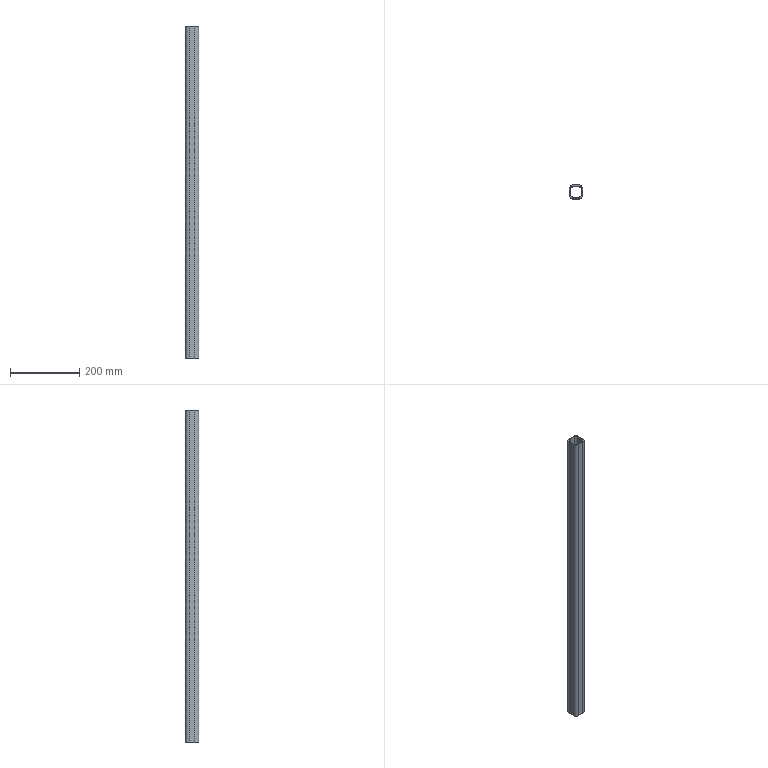Part | SolidWorks | features BaseBody 1 | 1 solid | 18 faces | box 40 x 40 x 962 mm | volume 488049 mm3 | plane 10 | cylinder 8 | commonest cylinder face diameters 16 x4 24 x4
STEP:
#1=CARTESIAN_POINT('',(8.,-20.,-50.));
#2=VERTEX_POINT('',#1);
#3=CARTESIAN_POINT('',(20.,-8.,-50.));
#4=VERTEX_POINT('',#3);
#5=CARTESIAN_POINT('',(8.,-8.,-50.));
#6=DIRECTION('',(0.,0.,1.));
#7=DIRECTION('',(1.,0.,0.));
#8=AXIS2_PLACEMENT_3D('',#5,#6,#7);
#9=CIRCLE('',#8,12.);
#10=EDGE_CURVE('',#2,#4,#9,.T.);
#11=ORIENTED_EDGE('',*,*,#10,.T.);
#12=CARTESIAN_POINT('',(20.,-8.,912.));
#13=VERTEX_POINT('',#12);
#14=CARTESIAN_POINT('',(20.,-8.,0.));
#15=DIRECTION('',(0.,0.,1.));
#16=VECTOR('',#15,1000.);
#17=LINE('',#14,#16);
#18=EDGE_CURVE('',#4,#13,#17,.T.);
#19=ORIENTED_EDGE('',*,*,#18,.T.);
#20=CARTESIAN_POINT('',(8.,-20.,912.));
#21=VERTEX_POINT('',#20);
#22=CARTESIAN_POINT('',(8.,-8.,912.));
#23=DIRECTION('',(0.,0.,-1.));
#24=DIRECTION('',(1.,0.,0.));
#25=AXIS2_PLACEMENT_3D('',#22,#23,#24);
#26=CIRCLE('',#25,12.);
#27=EDGE_CURVE('',#13,#21,#26,.T.);
#28=ORIENTED_EDGE('',*,*,#27,.T.);
#29=CARTESIAN_POINT('',(8.,-20.,0.));
#30=DIRECTION('',(0.,0.,-1.));
#31=VECTOR('',#30,1000.);
#32=LINE('',#29,#31);
#33=EDGE_CURVE('',#21,#2,#32,.T.);
#34=ORIENTED_EDGE('',*,*,#33,.T.);
#35=EDGE_LOOP('',(#11,#19,#28,#34));
#36=FACE_OUTER_BOUND('',#35,.T.);
#37=CARTESIAN_POINT('',(8.,-8.,0.));
#38=DIRECTION('',(0.,0.,1.));
#39=DIRECTION('',(1.,0.,0.));
#40=AXIS2_PLACEMENT_3D('',#37,#38,#39);
#41=CYLINDRICAL_SURFACE('',#40,12.);
#42=ADVANCED_FACE('',(#36),#41,.T.);
#43=CARTESIAN_POINT('',(20.,8.,-50.));
#44=VERTEX_POINT('',#43);
#45=CARTESIAN_POINT('',(20.,8.,-50.));
#46=DIRECTION('',(0.,1.,0.));
#47=VECTOR('',#46,1000.);
#48=LINE('',#45,#47);
#49=EDGE_CURVE('',#4,#44,#48,.T.);
#50=ORIENTED_EDGE('',*,*,#49,.T.);
#51=CARTESIAN_POINT('',(20.,8.,912.));
#52=VERTEX_POINT('',#51);
#53=CARTESIAN_POINT('',(20.,8.,0.));
#54=DIRECTION('',(0.,0.,1.));
#55=VECTOR('',#54,1000.);
#56=LINE('',#53,#55);
#57=EDGE_CURVE('',#44,#52,#56,.T.);
#58=ORIENTED_EDGE('',*,*,#57,.T.);
#59=CARTESIAN_POINT('',(20.,8.,912.));
#60=DIRECTION('',(0.,-1.,0.));
#61=VECTOR('',#60,1000.);
#62=LINE('',#59,#61);
#63=EDGE_CURVE('',#52,#13,#62,.T.);
#64=ORIENTED_EDGE('',*,*,#63,.T.);
#65=ORIENTED_EDGE('',*,*,#18,.F.);
#66=EDGE_LOOP('',(#50,#58,#64,#65));
#67=FACE_OUTER_BOUND('',#66,.T.);
#68=CARTESIAN_POINT('',(20.,8.,0.));
#69=DIRECTION('',(1.,0.,0.));
#70=DIRECTION('',(0.,1.,0.));
#71=AXIS2_PLACEMENT_3D('',#68,#69,#70);
#72=PLANE('',#71);
#73=ADVANCED_FACE('',(#67),#72,.T.);
#74=CARTESIAN_POINT('',(-16.,8.,-50.));
#75=VERTEX_POINT('',#74);
#76=CARTESIAN_POINT('',(-8.,16.,-50.));
#77=VERTEX_POINT('',#76);
#78=CARTESIAN_POINT('',(-8.,8.,-50.));
#79=DIRECTION('',(0.,0.,-1.));
#80=DIRECTION('',(1.,0.,0.));
#81=AXIS2_PLACEMENT_3D('',#78,#79,#80);
#82=CIRCLE('',#81,8.);
#83=EDGE_CURVE('',#75,#77,#82,.T.);
#84=ORIENTED_EDGE('',*,*,#83,.F.);
#85=CARTESIAN_POINT('',(-16.,-8.,-50.));
#86=VERTEX_POINT('',#85);
#87=CARTESIAN_POINT('',(-16.,0.,-50.));
#88=DIRECTION('',(0.,1.,0.));
#89=VECTOR('',#88,1000.);
#90=LINE('',#87,#89);
#91=EDGE_CURVE('',#86,#75,#90,.T.);
#92=ORIENTED_EDGE('',*,*,#91,.F.);
#93=CARTESIAN_POINT('',(-8.,-16.,-50.));
#94=VERTEX_POINT('',#93);
#95=CARTESIAN_POINT('',(-8.,-8.,-50.));
#96=DIRECTION('',(0.,0.,-1.));
#97=DIRECTION('',(1.,0.,0.));
#98=AXIS2_PLACEMENT_3D('',#95,#96,#97);
#99=CIRCLE('',#98,8.);
#100=EDGE_CURVE('',#94,#86,#99,.T.);
#101=ORIENTED_EDGE('',*,*,#100,.F.);
#102=CARTESIAN_POINT('',(8.,-16.,-50.));
#103=VERTEX_POINT('',#102);
#104=CARTESIAN_POINT('',(0.,-16.,-50.));
#105=DIRECTION('',(-1.,0.,0.));
#106=VECTOR('',#105,1000.);
#107=LINE('',#104,#106);
#108=EDGE_CURVE('',#103,#94,#107,.T.);
#109=ORIENTED_EDGE('',*,*,#108,.F.);
#110=CARTESIAN_POINT('',(16.,-8.,-50.));
#111=VERTEX_POINT('',#110);
#112=CARTESIAN_POINT('',(8.,-8.,-50.));
#113=DIRECTION('',(0.,0.,-1.));
#114=DIRECTION('',(1.,0.,0.));
#115=AXIS2_PLACEMENT_3D('',#112,#113,#114);
#116=CIRCLE('',#115,8.);
#117=EDGE_CURVE('',#111,#103,#116,.T.);
#118=ORIENTED_EDGE('',*,*,#117,.F.);
#119=CARTESIAN_POINT('',(16.,8.,-50.));
#120=VERTEX_POINT('',#119);
#121=CARTESIAN_POINT('',(16.,0.,-50.));
#122=DIRECTION('',(0.,-1.,0.));
#123=VECTOR('',#122,1000.);
#124=LINE('',#121,#123);
#125=EDGE_CURVE('',#120,#111,#124,.T.);
#126=ORIENTED_EDGE('',*,*,#125,.F.);
#127=CARTESIAN_POINT('',(8.,16.,-50.));
#128=VERTEX_POINT('',#127);
#129=CARTESIAN_POINT('',(8.,8.,-50.));
#130=DIRECTION('',(0.,0.,-1.));
#131=DIRECTION('',(1.,0.,0.));
#132=AXIS2_PLACEMENT_3D('',#129,#130,#131);
#133=CIRCLE('',#132,8.);
#134=EDGE_CURVE('',#128,#120,#133,.T.);
#135=ORIENTED_EDGE('',*,*,#134,.F.);
#136=CARTESIAN_POINT('',(0.,16.,-50.));
#137=DIRECTION('',(1.,0.,0.));
#138=VECTOR('',#137,1000.);
#139=LINE('',#136,#138);
#140=EDGE_CURVE('',#77,#128,#139,.T.);
#141=ORIENTED_EDGE('',*,*,#140,.F.);
#142=EDGE_LOOP('',(#84,#92,#101,#109,#118,#126,#135,#141));
#143=FACE_BOUND('',#142,.T.);
#144=CARTESIAN_POINT('',(-8.,20.,-50.));
#145=VERTEX_POINT('',#144);
#146=CARTESIAN_POINT('',(-20.,8.,-50.));
#147=VERTEX_POINT('',#146);
#148=CARTESIAN_POINT('',(-8.,8.,-50.));
#149=DIRECTION('',(0.,0.,1.));
#150=DIRECTION('',(1.,0.,0.));
#151=AXIS2_PLACEMENT_3D('',#148,#149,#150);
#152=CIRCLE('',#151,12.);
#153=EDGE_CURVE('',#145,#147,#152,.T.);
#154=ORIENTED_EDGE('',*,*,#153,.F.);
#155=CARTESIAN_POINT('',(8.,20.,-50.));
#156=VERTEX_POINT('',#155);
#157=CARTESIAN_POINT('',(0.,20.,-50.));
#158=DIRECTION('',(-1.,0.,0.));
#159=VECTOR('',#158,1000.);
#160=LINE('',#157,#159);
#161=EDGE_CURVE('',#156,#145,#160,.T.);
#162=ORIENTED_EDGE('',*,*,#161,.F.);
#163=CARTESIAN_POINT('',(8.,8.,-50.));
#164=DIRECTION('',(0.,0.,1.));
#165=DIRECTION('',(1.,0.,0.));
#166=AXIS2_PLACEMENT_3D('',#163,#164,#165);
#167=CIRCLE('',#166,12.);
#168=EDGE_CURVE('',#44,#156,#167,.T.);
#169=ORIENTED_EDGE('',*,*,#168,.F.);
#170=ORIENTED_EDGE('',*,*,#49,.F.);
#171=ORIENTED_EDGE('',*,*,#10,.F.);
#172=CARTESIAN_POINT('',(-8.,-20.,-50.));
#173=VERTEX_POINT('',#172);
#174=CARTESIAN_POINT('',(0.,-20.,-50.));
#175=DIRECTION('',(1.,0.,0.));
#176=VECTOR('',#175,1000.);
#177=LINE('',#174,#176);
#178=EDGE_CURVE('',#173,#2,#177,.T.);
#179=ORIENTED_EDGE('',*,*,#178,.F.);
#180=CARTESIAN_POINT('',(-20.,-8.,-50.));
#181=VERTEX_POINT('',#180);
#182=CARTESIAN_POINT('',(-8.,-8.,-50.));
#183=DIRECTION('',(0.,0.,1.));
#184=DIRECTION('',(1.,0.,0.));
#185=AXIS2_PLACEMENT_3D('',#182,#183,#184);
#186=CIRCLE('',#185,12.);
#187=EDGE_CURVE('',#181,#173,#186,.T.);
#188=ORIENTED_EDGE('',*,*,#187,.F.);
#189=CARTESIAN_POINT('',(-20.,0.,-50.));
#190=DIRECTION('',(0.,-1.,0.));
#191=VECTOR('',#190,1000.);
#192=LINE('',#189,#191);
#193=EDGE_CURVE('',#147,#181,#192,.T.);
#194=ORIENTED_EDGE('',*,*,#193,.F.);
#195=EDGE_LOOP('',(#154,#162,#169,#170,#171,#179,#188,#194));
#196=FACE_OUTER_BOUND('',#195,.T.);
#197=CARTESIAN_POINT('',(0.,0.,-50.));
#198=DIRECTION('',(0.,0.,1.));
#199=DIRECTION('',(1.,0.,0.));
#200=AXIS2_PLACEMENT_3D('',#197,#198,#199);
#201=PLANE('',#200);
#202=ADVANCED_FACE('',(#143,#196),#201,.F.);
#203=ORIENTED_EDGE('',*,*,#178,.T.);
#204=ORIENTED_EDGE('',*,*,#33,.F.);
#205=CARTESIAN_POINT('',(-8.,-20.,912.));
#206=VERTEX_POINT('',#205);
#207=CARTESIAN_POINT('',(8.,-20.,912.));
#208=DIRECTION('',(-1.,0.,0.));
#209=VECTOR('',#208,1000.);
#210=LINE('',#207,#209);
#211=EDGE_CURVE('',#21,#206,#210,.T.);
#212=ORIENTED_EDGE('',*,*,#211,.T.);
#213=CARTESIAN_POINT('',(-8.,-20.,0.));
#214=DIRECTION('',(0.,0.,-1.));
#215=VECTOR('',#214,1000.);
#216=LINE('',#213,#215);
#217=EDGE_CURVE('',#206,#173,#216,.T.);
#218=ORIENTED_EDGE('',*,*,#217,.T.);
#219=EDGE_LOOP('',(#203,#204,#212,#218));
#220=FACE_OUTER_BOUND('',#219,.T.);
#221=CARTESIAN_POINT('',(8.,-20.,0.));
#222=DIRECTION('',(0.,-1.,0.));
#223=DIRECTION('',(1.,0.,0.));
#224=AXIS2_PLACEMENT_3D('',#221,#222,#223);
#225=PLANE('',#224);
#226=ADVANCED_FACE('',(#220),#225,.T.);
#227=CARTESIAN_POINT('',(-16.,-8.,912.));
#228=VERTEX_POINT('',#227);
#229=CARTESIAN_POINT('',(-16.,8.,912.));
#230=VERTEX_POINT('',#229);
#231=CARTESIAN_POINT('',(-16.,0.,912.));
#232=DIRECTION('',(0.,1.,0.));
#233=VECTOR('',#232,1000.);
#234=LINE('',#231,#233);
#235=EDGE_CURVE('',#228,#230,#234,.T.);
#236=ORIENTED_EDGE('',*,*,#235,.T.);
#237=CARTESIAN_POINT('',(-8.,16.,912.));
#238=VERTEX_POINT('',#237);
#239=CARTESIAN_POINT('',(-8.,8.,912.));
#240=DIRECTION('',(0.,0.,-1.));
#241=DIRECTION('',(1.,0.,0.));
#242=AXIS2_PLACEMENT_3D('',#239,#240,#241);
#243=CIRCLE('',#242,8.);
#244=EDGE_CURVE('',#230,#238,#243,.T.);
#245=ORIENTED_EDGE('',*,*,#244,.T.);
#246=CARTESIAN_POINT('',(8.,16.,912.));
#247=VERTEX_POINT('',#246);
#248=CARTESIAN_POINT('',(0.,16.,912.));
#249=DIRECTION('',(1.,0.,0.));
#250=VECTOR('',#249,1000.);
#251=LINE('',#248,#250);
#252=EDGE_CURVE('',#238,#247,#251,.T.);
#253=ORIENTED_EDGE('',*,*,#252,.T.);
#254=CARTESIAN_POINT('',(16.,8.,912.));
#255=VERTEX_POINT('',#254);
#256=CARTESIAN_POINT('',(8.,8.,912.));
#257=DIRECTION('',(0.,0.,-1.));
#258=DIRECTION('',(1.,0.,0.));
#259=AXIS2_PLACEMENT_3D('',#256,#257,#258);
#260=CIRCLE('',#259,8.);
#261=EDGE_CURVE('',#247,#255,#260,.T.);
#262=ORIENTED_EDGE('',*,*,#261,.T.);
#263=CARTESIAN_POINT('',(16.,-8.,912.));
#264=VERTEX_POINT('',#263);
#265=CARTESIAN_POINT('',(16.,0.,912.));
#266=DIRECTION('',(0.,-1.,0.));
#267=VECTOR('',#266,1000.);
#268=LINE('',#265,#267);
#269=EDGE_CURVE('',#255,#264,#268,.T.);
#270=ORIENTED_EDGE('',*,*,#269,.T.);
#271=CARTESIAN_POINT('',(8.,-16.,912.));
#272=VERTEX_POINT('',#271);
#273=CARTESIAN_POINT('',(8.,-8.,912.));
#274=DIRECTION('',(0.,0.,-1.));
#275=DIRECTION('',(1.,0.,0.));
#276=AXIS2_PLACEMENT_3D('',#273,#274,#275);
#277=CIRCLE('',#276,8.);
#278=EDGE_CURVE('',#264,#272,#277,.T.);
#279=ORIENTED_EDGE('',*,*,#278,.T.);
#280=CARTESIAN_POINT('',(-8.,-16.,912.));
#281=VERTEX_POINT('',#280);
#282=CARTESIAN_POINT('',(0.,-16.,912.));
#283=DIRECTION('',(-1.,0.,0.));
#284=VECTOR('',#283,1000.);
#285=LINE('',#282,#284);
#286=EDGE_CURVE('',#272,#281,#285,.T.);
#287=ORIENTED_EDGE('',*,*,#286,.T.);
#288=CARTESIAN_POINT('',(-8.,-8.,912.));
#289=DIRECTION('',(0.,0.,-1.));
#290=DIRECTION('',(1.,0.,0.));
#291=AXIS2_PLACEMENT_3D('',#288,#289,#290);
#292=CIRCLE('',#291,8.);
#293=EDGE_CURVE('',#281,#228,#292,.T.);
#294=ORIENTED_EDGE('',*,*,#293,.T.);
#295=EDGE_LOOP('',(#236,#245,#253,#262,#270,#279,#287,#294));
#296=FACE_BOUND('',#295,.T.);
#297=CARTESIAN_POINT('',(8.,20.,912.));
#298=VERTEX_POINT('',#297);
#299=CARTESIAN_POINT('',(-8.,20.,912.));
#300=VERTEX_POINT('',#299);
#301=CARTESIAN_POINT('',(0.,20.,912.));
#302=DIRECTION('',(-1.,0.,0.));
#303=VECTOR('',#302,1000.);
#304=LINE('',#301,#303);
#305=EDGE_CURVE('',#298,#300,#304,.T.);
#306=ORIENTED_EDGE('',*,*,#305,.T.);
#307=CARTESIAN_POINT('',(-20.,8.,912.));
#308=VERTEX_POINT('',#307);
#309=CARTESIAN_POINT('',(-8.,8.,912.));
#310=DIRECTION('',(0.,0.,1.));
#311=DIRECTION('',(1.,0.,0.));
#312=AXIS2_PLACEMENT_3D('',#309,#310,#311);
#313=CIRCLE('',#312,12.);
#314=EDGE_CURVE('',#300,#308,#313,.T.);
#315=ORIENTED_EDGE('',*,*,#314,.T.);
#316=CARTESIAN_POINT('',(-20.,-8.,912.));
#317=VERTEX_POINT('',#316);
#318=CARTESIAN_POINT('',(-20.,0.,912.));
#319=DIRECTION('',(0.,-1.,0.));
#320=VECTOR('',#319,1000.);
#321=LINE('',#318,#320);
#322=EDGE_CURVE('',#308,#317,#321,.T.);
#323=ORIENTED_EDGE('',*,*,#322,.T.);
#324=CARTESIAN_POINT('',(-8.,-8.,912.));
#325=DIRECTION('',(0.,0.,1.));
#326=DIRECTION('',(1.,0.,0.));
#327=AXIS2_PLACEMENT_3D('',#324,#325,#326);
#328=CIRCLE('',#327,12.);
#329=EDGE_CURVE('',#317,#206,#328,.T.);
#330=ORIENTED_EDGE('',*,*,#329,.T.);
#331=ORIENTED_EDGE('',*,*,#211,.F.);
#332=ORIENTED_EDGE('',*,*,#27,.F.);
#333=ORIENTED_EDGE('',*,*,#63,.F.);
#334=CARTESIAN_POINT('',(8.,8.,912.));
#335=DIRECTION('',(0.,0.,1.));
#336=DIRECTION('',(1.,0.,0.));
#337=AXIS2_PLACEMENT_3D('',#334,#335,#336);
#338=CIRCLE('',#337,12.);
#339=EDGE_CURVE('',#52,#298,#338,.T.);
#340=ORIENTED_EDGE('',*,*,#339,.T.);
#341=EDGE_LOOP('',(#306,#315,#323,#330,#331,#332,#333,#340));
#342=FACE_OUTER_BOUND('',#341,.T.);
#343=CARTESIAN_POINT('',(0.,0.,912.));
#344=DIRECTION('',(0.,0.,1.));
#345=DIRECTION('',(1.,0.,0.));
#346=AXIS2_PLACEMENT_3D('',#343,#344,#345);
#347=PLANE('',#346);
#348=ADVANCED_FACE('',(#296,#342),#347,.T.);
#349=ORIENTED_EDGE('',*,*,#168,.T.);
#350=CARTESIAN_POINT('',(8.,20.,0.));
#351=DIRECTION('',(0.,0.,1.));
#352=VECTOR('',#351,1000.);
#353=LINE('',#350,#352);
#354=EDGE_CURVE('',#156,#298,#353,.T.);
#355=ORIENTED_EDGE('',*,*,#354,.T.);
#356=ORIENTED_EDGE('',*,*,#339,.F.);
#357=ORIENTED_EDGE('',*,*,#57,.F.);
#358=EDGE_LOOP('',(#349,#355,#356,#357));
#359=FACE_OUTER_BOUND('',#358,.T.);
#360=CARTESIAN_POINT('',(8.,8.,0.));
#361=DIRECTION('',(0.,0.,1.));
#362=DIRECTION('',(1.,0.,0.));
#363=AXIS2_PLACEMENT_3D('',#360,#361,#362);
#364=CYLINDRICAL_SURFACE('',#363,12.);
#365=ADVANCED_FACE('',(#359),#364,.T.);
#366=CARTESIAN_POINT('',(-8.,16.,0.));
#367=DIRECTION('',(0.,0.,1.));
#368=VECTOR('',#367,1000.);
#369=LINE('',#366,#368);
#370=EDGE_CURVE('',#77,#238,#369,.T.);
#371=ORIENTED_EDGE('',*,*,#370,.F.);
#372=ORIENTED_EDGE('',*,*,#140,.T.);
#373=CARTESIAN_POINT('',(8.,16.,0.));
#374=DIRECTION('',(0.,0.,-1.));
#375=VECTOR('',#374,1000.);
#376=LINE('',#373,#375);
#377=EDGE_CURVE('',#247,#128,#376,.T.);
#378=ORIENTED_EDGE('',*,*,#377,.F.);
#379=ORIENTED_EDGE('',*,*,#252,.F.);
#380=EDGE_LOOP('',(#371,#372,#378,#379));
#381=FACE_OUTER_BOUND('',#380,.T.);
#382=CARTESIAN_POINT('',(-8.,16.,0.));
#383=DIRECTION('',(0.,1.,0.));
#384=DIRECTION('',(-1.,0.,0.));
#385=AXIS2_PLACEMENT_3D('',#382,#383,#384);
#386=PLANE('',#385);
#387=ADVANCED_FACE('',(#381),#386,.F.);
#388=CARTESIAN_POINT('',(-16.,8.,0.));
#389=DIRECTION('',(0.,0.,1.));
#390=VECTOR('',#389,1000.);
#391=LINE('',#388,#390);
#392=EDGE_CURVE('',#75,#230,#391,.T.);
#393=ORIENTED_EDGE('',*,*,#392,.F.);
#394=ORIENTED_EDGE('',*,*,#83,.T.);
#395=ORIENTED_EDGE('',*,*,#370,.T.);
#396=ORIENTED_EDGE('',*,*,#244,.F.);
#397=EDGE_LOOP('',(#393,#394,#395,#396));
#398=FACE_OUTER_BOUND('',#397,.T.);
#399=CARTESIAN_POINT('',(-8.,8.,0.));
#400=DIRECTION('',(0.,0.,1.));
#401=DIRECTION('',(1.,0.,0.));
#402=AXIS2_PLACEMENT_3D('',#399,#400,#401);
#403=CYLINDRICAL_SURFACE('',#402,8.);
#404=ADVANCED_FACE('',(#398),#403,.F.);
#405=CARTESIAN_POINT('',(-16.,-8.,0.));
#406=DIRECTION('',(0.,0.,1.));
#407=VECTOR('',#406,1000.);
#408=LINE('',#405,#407);
#409=EDGE_CURVE('',#86,#228,#408,.T.);
#410=ORIENTED_EDGE('',*,*,#409,.F.);
#411=ORIENTED_EDGE('',*,*,#91,.T.);
#412=ORIENTED_EDGE('',*,*,#392,.T.);
#413=ORIENTED_EDGE('',*,*,#235,.F.);
#414=EDGE_LOOP('',(#410,#411,#412,#413));
#415=FACE_OUTER_BOUND('',#414,.T.);
#416=CARTESIAN_POINT('',(-16.,-8.,0.));
#417=DIRECTION('',(-1.,0.,0.));
#418=DIRECTION('',(0.,-1.,0.));
#419=AXIS2_PLACEMENT_3D('',#416,#417,#418);
#420=PLANE('',#419);
#421=ADVANCED_FACE('',(#415),#420,.F.);
#422=CARTESIAN_POINT('',(-8.,-16.,0.));
#423=DIRECTION('',(0.,0.,1.));
#424=VECTOR('',#423,1000.);
#425=LINE('',#422,#424);
#426=EDGE_CURVE('',#94,#281,#425,.T.);
#427=ORIENTED_EDGE('',*,*,#426,.F.);
#428=ORIENTED_EDGE('',*,*,#100,.T.);
#429=ORIENTED_EDGE('',*,*,#409,.T.);
#430=ORIENTED_EDGE('',*,*,#293,.F.);
#431=EDGE_LOOP('',(#427,#428,#429,#430));
#432=FACE_OUTER_BOUND('',#431,.T.);
#433=CARTESIAN_POINT('',(-8.,-8.,0.));
#434=DIRECTION('',(0.,0.,1.));
#435=DIRECTION('',(1.,0.,0.));
#436=AXIS2_PLACEMENT_3D('',#433,#434,#435);
#437=CYLINDRICAL_SURFACE('',#436,8.);
#438=ADVANCED_FACE('',(#432),#437,.F.);
#439=CARTESIAN_POINT('',(8.,-16.,0.));
#440=DIRECTION('',(0.,0.,1.));
#441=VECTOR('',#440,1000.);
#442=LINE('',#439,#441);
#443=EDGE_CURVE('',#103,#272,#442,.T.);
#444=ORIENTED_EDGE('',*,*,#443,.F.);
#445=ORIENTED_EDGE('',*,*,#108,.T.);
#446=ORIENTED_EDGE('',*,*,#426,.T.);
#447=ORIENTED_EDGE('',*,*,#286,.F.);
#448=EDGE_LOOP('',(#444,#445,#446,#447));
#449=FACE_OUTER_BOUND('',#448,.T.);
#450=CARTESIAN_POINT('',(8.,-16.,0.));
#451=DIRECTION('',(0.,-1.,0.));
#452=DIRECTION('',(1.,0.,0.));
#453=AXIS2_PLACEMENT_3D('',#450,#451,#452);
#454=PLANE('',#453);
#455=ADVANCED_FACE('',(#449),#454,.F.);
#456=CARTESIAN_POINT('',(16.,-8.,0.));
#457=DIRECTION('',(0.,0.,1.));
#458=VECTOR('',#457,1000.);
#459=LINE('',#456,#458);
#460=EDGE_CURVE('',#111,#264,#459,.T.);
#461=ORIENTED_EDGE('',*,*,#460,.F.);
#462=ORIENTED_EDGE('',*,*,#117,.T.);
#463=ORIENTED_EDGE('',*,*,#443,.T.);
#464=ORIENTED_EDGE('',*,*,#278,.F.);
#465=EDGE_LOOP('',(#461,#462,#463,#464));
#466=FACE_OUTER_BOUND('',#465,.T.);
#467=CARTESIAN_POINT('',(8.,-8.,0.));
#468=DIRECTION('',(0.,0.,1.));
#469=DIRECTION('',(1.,0.,0.));
#470=AXIS2_PLACEMENT_3D('',#467,#468,#469);
#471=CYLINDRICAL_SURFACE('',#470,8.);
#472=ADVANCED_FACE('',(#466),#471,.F.);
#473=CARTESIAN_POINT('',(16.,8.,0.));
#474=DIRECTION('',(0.,0.,1.));
#475=VECTOR('',#474,1000.);
#476=LINE('',#473,#475);
#477=EDGE_CURVE('',#120,#255,#476,.T.);
#478=ORIENTED_EDGE('',*,*,#477,.F.);
#479=ORIENTED_EDGE('',*,*,#125,.T.);
#480=ORIENTED_EDGE('',*,*,#460,.T.);
#481=ORIENTED_EDGE('',*,*,#269,.F.);
#482=EDGE_LOOP('',(#478,#479,#480,#481));
#483=FACE_OUTER_BOUND('',#482,.T.);
#484=CARTESIAN_POINT('',(16.,8.,0.));
#485=DIRECTION('',(1.,0.,0.));
#486=DIRECTION('',(0.,0.,-1.));
#487=AXIS2_PLACEMENT_3D('',#484,#485,#486);
#488=PLANE('',#487);
#489=ADVANCED_FACE('',(#483),#488,.F.);
#490=ORIENTED_EDGE('',*,*,#377,.T.);
#491=ORIENTED_EDGE('',*,*,#134,.T.);
#492=ORIENTED_EDGE('',*,*,#477,.T.);
#493=ORIENTED_EDGE('',*,*,#261,.F.);
#494=EDGE_LOOP('',(#490,#491,#492,#493));
#495=FACE_OUTER_BOUND('',#494,.T.);
#496=CARTESIAN_POINT('',(8.,8.,0.));
#497=DIRECTION('',(0.,0.,1.));
#498=DIRECTION('',(1.,0.,0.));
#499=AXIS2_PLACEMENT_3D('',#496,#497,#498);
#500=CYLINDRICAL_SURFACE('',#499,8.);
#501=ADVANCED_FACE('',(#495),#500,.F.);
#502=ORIENTED_EDGE('',*,*,#193,.T.);
#503=CARTESIAN_POINT('',(-20.,-8.,0.));
#504=DIRECTION('',(0.,0.,1.));
#505=VECTOR('',#504,1000.);
#506=LINE('',#503,#505);
#507=EDGE_CURVE('',#181,#317,#506,.T.);
#508=ORIENTED_EDGE('',*,*,#507,.T.);
#509=ORIENTED_EDGE('',*,*,#322,.F.);
#510=CARTESIAN_POINT('',(-20.,8.,0.));
#511=DIRECTION('',(0.,0.,-1.));
#512=VECTOR('',#511,1000.);
#513=LINE('',#510,#512);
#514=EDGE_CURVE('',#308,#147,#513,.T.);
#515=ORIENTED_EDGE('',*,*,#514,.T.);
#516=EDGE_LOOP('',(#502,#508,#509,#515));
#517=FACE_OUTER_BOUND('',#516,.T.);
#518=CARTESIAN_POINT('',(-20.,-8.,0.));
#519=DIRECTION('',(-1.,0.,0.));
#520=DIRECTION('',(0.,-1.,0.));
#521=AXIS2_PLACEMENT_3D('',#518,#519,#520);
#522=PLANE('',#521);
#523=ADVANCED_FACE('',(#517),#522,.T.);
#524=ORIENTED_EDGE('',*,*,#153,.T.);
#525=ORIENTED_EDGE('',*,*,#514,.F.);
#526=ORIENTED_EDGE('',*,*,#314,.F.);
#527=CARTESIAN_POINT('',(-8.,20.,0.));
#528=DIRECTION('',(0.,0.,-1.));
#529=VECTOR('',#528,1000.);
#530=LINE('',#527,#529);
#531=EDGE_CURVE('',#300,#145,#530,.T.);
#532=ORIENTED_EDGE('',*,*,#531,.T.);
#533=EDGE_LOOP('',(#524,#525,#526,#532));
#534=FACE_OUTER_BOUND('',#533,.T.);
#535=CARTESIAN_POINT('',(-8.,8.,0.));
#536=DIRECTION('',(0.,0.,1.));
#537=DIRECTION('',(1.,0.,0.));
#538=AXIS2_PLACEMENT_3D('',#535,#536,#537);
#539=CYLINDRICAL_SURFACE('',#538,12.);
#540=ADVANCED_FACE('',(#534),#539,.T.);
#541=ORIENTED_EDGE('',*,*,#161,.T.);
#542=ORIENTED_EDGE('',*,*,#531,.F.);
#543=ORIENTED_EDGE('',*,*,#305,.F.);
#544=ORIENTED_EDGE('',*,*,#354,.F.);
#545=EDGE_LOOP('',(#541,#542,#543,#544));
#546=FACE_OUTER_BOUND('',#545,.T.);
#547=CARTESIAN_POINT('',(-8.,20.,0.));
#548=DIRECTION('',(0.,1.,0.));
#549=DIRECTION('',(0.,0.,1.));
#550=AXIS2_PLACEMENT_3D('',#547,#548,#549);
#551=PLANE('',#550);
#552=ADVANCED_FACE('',(#546),#551,.T.);
#553=ORIENTED_EDGE('',*,*,#187,.T.);
#554=ORIENTED_EDGE('',*,*,#217,.F.);
#555=ORIENTED_EDGE('',*,*,#329,.F.);
#556=ORIENTED_EDGE('',*,*,#507,.F.);
#557=EDGE_LOOP('',(#553,#554,#555,#556));
#558=FACE_OUTER_BOUND('',#557,.T.);
#559=CARTESIAN_POINT('',(-8.,-8.,0.));
#560=DIRECTION('',(0.,0.,1.));
#561=DIRECTION('',(1.,0.,0.));
#562=AXIS2_PLACEMENT_3D('',#559,#560,#561);
#563=CYLINDRICAL_SURFACE('',#562,12.);
#564=ADVANCED_FACE('',(#558),#563,.T.);
#565=CLOSED_SHELL('',(#42,#73,#202,#226,#348,#365,#387,#404,#421,#438,#455,#472,#489,#501,#523,#540,#552,#564));
#566=MANIFOLD_SOLID_BREP('',#565);
#567=CARTESIAN_POINT('',(0.,0.,0.));
#568=DIRECTION('',(0.,0.,1.));
#569=DIRECTION('',(1.,0.,0.));
#570=AXIS2_PLACEMENT_3D('',#567,#568,#569);
#571=(LENGTH_UNIT()NAMED_UNIT(*)SI_UNIT(.MILLI.,.METRE.));
#572=UNCERTAINTY_MEASURE_WITH_UNIT(LENGTH_MEASURE(0.00001),#571,'','');
#573=(NAMED_UNIT(*)PLANE_ANGLE_UNIT()SI_UNIT($,.RADIAN.));
#574=(NAMED_UNIT(*)SI_UNIT($,.STERADIAN.)SOLID_ANGLE_UNIT());
#575=(GEOMETRIC_REPRESENTATION_CONTEXT(3)GLOBAL_UNCERTAINTY_ASSIGNED_CONTEXT((#572))GLOBAL_UNIT_ASSIGNED_CONTEXT((#571,#573,#574))REPRESENTATION_CONTEXT('',''));
#576=ADVANCED_BREP_SHAPE_REPRESENTATION('',(#566,#570),#575);